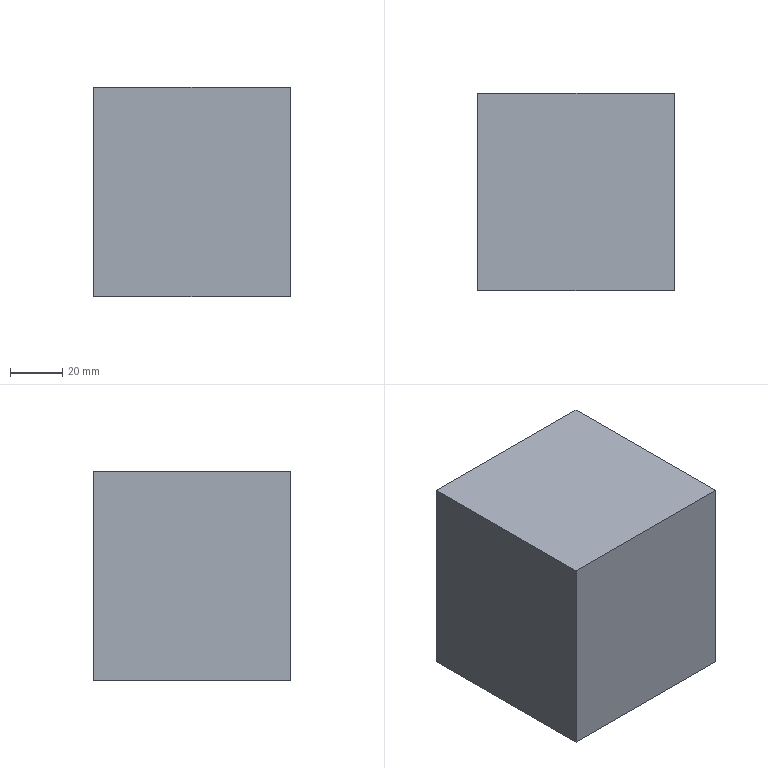Part | SolidWorks | features Extrusion 1, HoleWzd 1 | 1 solid | 30 faces | box 75 x 75 x 80 mm | volume 448174 mm3 | cylinder 12 | cone 12 | plane 6 | commonest cylinder face diameters 5 x12
STEP:
#1=CARTESIAN_POINT('',(34.,31.,15.));
#2=VERTEX_POINT('',#1);
#3=CARTESIAN_POINT('',(29.,31.,15.));
#4=VERTEX_POINT('',#3);
#5=CARTESIAN_POINT('',(31.5,31.,15.));
#6=DIRECTION('',(0.,0.,-1.));
#7=DIRECTION('',(-1.,0.,0.));
#8=AXIS2_PLACEMENT_3D('',#5,#6,#7);
#9=CIRCLE('',#8,2.5);
#10=EDGE_CURVE('',#2,#4,#9,.T.);
#11=ORIENTED_EDGE('',*,*,#10,.F.);
#12=CARTESIAN_POINT('',(34.,31.,0.));
#13=VERTEX_POINT('',#12);
#14=CARTESIAN_POINT('',(34.,31.,0.));
#15=DIRECTION('',(0.,0.,-1.));
#16=VECTOR('',#15,1000.);
#17=LINE('',#14,#16);
#18=EDGE_CURVE('',#2,#13,#17,.T.);
#19=ORIENTED_EDGE('',*,*,#18,.T.);
#20=CARTESIAN_POINT('',(29.,31.,0.));
#21=VERTEX_POINT('',#20);
#22=CARTESIAN_POINT('',(31.5,31.,0.));
#23=DIRECTION('',(0.,0.,-1.));
#24=DIRECTION('',(-1.,0.,0.));
#25=AXIS2_PLACEMENT_3D('',#22,#23,#24);
#26=CIRCLE('',#25,2.5);
#27=EDGE_CURVE('',#13,#21,#26,.T.);
#28=ORIENTED_EDGE('',*,*,#27,.T.);
#29=CARTESIAN_POINT('',(29.,31.,0.));
#30=DIRECTION('',(0.,0.,-1.));
#31=VECTOR('',#30,1000.);
#32=LINE('',#29,#31);
#33=EDGE_CURVE('',#4,#21,#32,.T.);
#34=ORIENTED_EDGE('',*,*,#33,.F.);
#35=EDGE_LOOP('',(#11,#19,#28,#34));
#36=FACE_OUTER_BOUND('',#35,.T.);
#37=CARTESIAN_POINT('',(31.5,31.,0.));
#38=DIRECTION('',(0.,0.,-1.));
#39=DIRECTION('',(-1.,0.,0.));
#40=AXIS2_PLACEMENT_3D('',#37,#38,#39);
#41=CYLINDRICAL_SURFACE('',#40,2.5);
#42=ADVANCED_FACE('',(#36),#41,.F.);
#43=CARTESIAN_POINT('',(31.5,31.,16.502));
#44=VERTEX_POINT('',#43);
#45=CARTESIAN_POINT('',(29.,31.,15.));
#46=DIRECTION('',(-0.8572,0.,-0.515));
#47=VECTOR('',#46,1000.);
#48=LINE('',#45,#47);
#49=EDGE_CURVE('',#44,#4,#48,.T.);
#50=ORIENTED_EDGE('',*,*,#49,.F.);
#51=CARTESIAN_POINT('',(34.,31.,15.));
#52=DIRECTION('',(0.8572,0.,-0.515));
#53=VECTOR('',#52,1000.);
#54=LINE('',#51,#53);
#55=EDGE_CURVE('',#44,#2,#54,.T.);
#56=ORIENTED_EDGE('',*,*,#55,.T.);
#57=ORIENTED_EDGE('',*,*,#10,.T.);
#58=EDGE_LOOP('',(#50,#56,#57));
#59=FACE_OUTER_BOUND('',#58,.T.);
#60=CARTESIAN_POINT('',(31.5,31.,15.));
#61=DIRECTION('',(0.,0.,-1.));
#62=DIRECTION('',(-1.,0.,0.));
#63=AXIS2_PLACEMENT_3D('',#60,#61,#62);
#64=CONICAL_SURFACE('',#63,2.5,1.03);
#65=ADVANCED_FACE('',(#59),#64,.F.);
#66=CARTESIAN_POINT('',(23.,31.,15.));
#67=VERTEX_POINT('',#66);
#68=CARTESIAN_POINT('',(18.,31.,15.));
#69=VERTEX_POINT('',#68);
#70=CARTESIAN_POINT('',(20.5,31.,15.));
#71=DIRECTION('',(0.,0.,-1.));
#72=DIRECTION('',(-1.,0.,0.));
#73=AXIS2_PLACEMENT_3D('',#70,#71,#72);
#74=CIRCLE('',#73,2.5);
#75=EDGE_CURVE('',#67,#69,#74,.T.);
#76=ORIENTED_EDGE('',*,*,#75,.F.);
#77=CARTESIAN_POINT('',(23.,31.,0.));
#78=VERTEX_POINT('',#77);
#79=CARTESIAN_POINT('',(23.,31.,0.));
#80=DIRECTION('',(0.,0.,-1.));
#81=VECTOR('',#80,1000.);
#82=LINE('',#79,#81);
#83=EDGE_CURVE('',#67,#78,#82,.T.);
#84=ORIENTED_EDGE('',*,*,#83,.T.);
#85=CARTESIAN_POINT('',(18.,31.,0.));
#86=VERTEX_POINT('',#85);
#87=CARTESIAN_POINT('',(20.5,31.,0.));
#88=DIRECTION('',(0.,0.,-1.));
#89=DIRECTION('',(-1.,0.,0.));
#90=AXIS2_PLACEMENT_3D('',#87,#88,#89);
#91=CIRCLE('',#90,2.5);
#92=EDGE_CURVE('',#78,#86,#91,.T.);
#93=ORIENTED_EDGE('',*,*,#92,.T.);
#94=CARTESIAN_POINT('',(18.,31.,0.));
#95=DIRECTION('',(0.,0.,-1.));
#96=VECTOR('',#95,1000.);
#97=LINE('',#94,#96);
#98=EDGE_CURVE('',#69,#86,#97,.T.);
#99=ORIENTED_EDGE('',*,*,#98,.F.);
#100=EDGE_LOOP('',(#76,#84,#93,#99));
#101=FACE_OUTER_BOUND('',#100,.T.);
#102=CARTESIAN_POINT('',(20.5,31.,0.));
#103=DIRECTION('',(0.,0.,-1.));
#104=DIRECTION('',(-1.,0.,0.));
#105=AXIS2_PLACEMENT_3D('',#102,#103,#104);
#106=CYLINDRICAL_SURFACE('',#105,2.5);
#107=ADVANCED_FACE('',(#101),#106,.F.);
#108=CARTESIAN_POINT('',(20.5,31.,16.502));
#109=VERTEX_POINT('',#108);
#110=CARTESIAN_POINT('',(18.,31.,15.));
#111=DIRECTION('',(-0.8572,0.,-0.515));
#112=VECTOR('',#111,1000.);
#113=LINE('',#110,#112);
#114=EDGE_CURVE('',#109,#69,#113,.T.);
#115=ORIENTED_EDGE('',*,*,#114,.F.);
#116=CARTESIAN_POINT('',(23.,31.,15.));
#117=DIRECTION('',(0.8572,0.,-0.515));
#118=VECTOR('',#117,1000.);
#119=LINE('',#116,#118);
#120=EDGE_CURVE('',#109,#67,#119,.T.);
#121=ORIENTED_EDGE('',*,*,#120,.T.);
#122=ORIENTED_EDGE('',*,*,#75,.T.);
#123=EDGE_LOOP('',(#115,#121,#122));
#124=FACE_OUTER_BOUND('',#123,.T.);
#125=CARTESIAN_POINT('',(20.5,31.,15.));
#126=DIRECTION('',(0.,0.,-1.));
#127=DIRECTION('',(-1.,0.,0.));
#128=AXIS2_PLACEMENT_3D('',#125,#126,#127);
#129=CONICAL_SURFACE('',#128,2.5,1.03);
#130=ADVANCED_FACE('',(#124),#129,.F.);
#131=CARTESIAN_POINT('',(-18.,31.,15.));
#132=VERTEX_POINT('',#131);
#133=CARTESIAN_POINT('',(-23.,31.,15.));
#134=VERTEX_POINT('',#133);
#135=CARTESIAN_POINT('',(-20.5,31.,15.));
#136=DIRECTION('',(0.,0.,-1.));
#137=DIRECTION('',(-1.,0.,0.));
#138=AXIS2_PLACEMENT_3D('',#135,#136,#137);
#139=CIRCLE('',#138,2.5);
#140=EDGE_CURVE('',#132,#134,#139,.T.);
#141=ORIENTED_EDGE('',*,*,#140,.F.);
#142=CARTESIAN_POINT('',(-18.,31.,0.));
#143=VERTEX_POINT('',#142);
#144=CARTESIAN_POINT('',(-18.,31.,0.));
#145=DIRECTION('',(0.,0.,-1.));
#146=VECTOR('',#145,1000.);
#147=LINE('',#144,#146);
#148=EDGE_CURVE('',#132,#143,#147,.T.);
#149=ORIENTED_EDGE('',*,*,#148,.T.);
#150=CARTESIAN_POINT('',(-23.,31.,0.));
#151=VERTEX_POINT('',#150);
#152=CARTESIAN_POINT('',(-20.5,31.,0.));
#153=DIRECTION('',(0.,0.,-1.));
#154=DIRECTION('',(-1.,0.,0.));
#155=AXIS2_PLACEMENT_3D('',#152,#153,#154);
#156=CIRCLE('',#155,2.5);
#157=EDGE_CURVE('',#143,#151,#156,.T.);
#158=ORIENTED_EDGE('',*,*,#157,.T.);
#159=CARTESIAN_POINT('',(-23.,31.,0.));
#160=DIRECTION('',(0.,0.,-1.));
#161=VECTOR('',#160,1000.);
#162=LINE('',#159,#161);
#163=EDGE_CURVE('',#134,#151,#162,.T.);
#164=ORIENTED_EDGE('',*,*,#163,.F.);
#165=EDGE_LOOP('',(#141,#149,#158,#164));
#166=FACE_OUTER_BOUND('',#165,.T.);
#167=CARTESIAN_POINT('',(-20.5,31.,0.));
#168=DIRECTION('',(0.,0.,-1.));
#169=DIRECTION('',(-1.,0.,0.));
#170=AXIS2_PLACEMENT_3D('',#167,#168,#169);
#171=CYLINDRICAL_SURFACE('',#170,2.5);
#172=ADVANCED_FACE('',(#166),#171,.F.);
#173=CARTESIAN_POINT('',(-20.5,31.,16.502));
#174=VERTEX_POINT('',#173);
#175=CARTESIAN_POINT('',(-23.,31.,15.));
#176=DIRECTION('',(-0.8572,0.,-0.515));
#177=VECTOR('',#176,1000.);
#178=LINE('',#175,#177);
#179=EDGE_CURVE('',#174,#134,#178,.T.);
#180=ORIENTED_EDGE('',*,*,#179,.F.);
#181=CARTESIAN_POINT('',(-18.,31.,15.));
#182=DIRECTION('',(0.8572,0.,-0.515));
#183=VECTOR('',#182,1000.);
#184=LINE('',#181,#183);
#185=EDGE_CURVE('',#174,#132,#184,.T.);
#186=ORIENTED_EDGE('',*,*,#185,.T.);
#187=ORIENTED_EDGE('',*,*,#140,.T.);
#188=EDGE_LOOP('',(#180,#186,#187));
#189=FACE_OUTER_BOUND('',#188,.T.);
#190=CARTESIAN_POINT('',(-20.5,31.,15.));
#191=DIRECTION('',(0.,0.,-1.));
#192=DIRECTION('',(-1.,0.,0.));
#193=AXIS2_PLACEMENT_3D('',#190,#191,#192);
#194=CONICAL_SURFACE('',#193,2.5,1.03);
#195=ADVANCED_FACE('',(#189),#194,.F.);
#196=CARTESIAN_POINT('',(-18.,-31.,15.));
#197=VERTEX_POINT('',#196);
#198=CARTESIAN_POINT('',(-23.,-31.,15.));
#199=VERTEX_POINT('',#198);
#200=CARTESIAN_POINT('',(-20.5,-31.,15.));
#201=DIRECTION('',(0.,0.,-1.));
#202=DIRECTION('',(-1.,0.,0.));
#203=AXIS2_PLACEMENT_3D('',#200,#201,#202);
#204=CIRCLE('',#203,2.5);
#205=EDGE_CURVE('',#197,#199,#204,.T.);
#206=ORIENTED_EDGE('',*,*,#205,.F.);
#207=CARTESIAN_POINT('',(-18.,-31.,0.));
#208=VERTEX_POINT('',#207);
#209=CARTESIAN_POINT('',(-18.,-31.,0.));
#210=DIRECTION('',(0.,0.,-1.));
#211=VECTOR('',#210,1000.);
#212=LINE('',#209,#211);
#213=EDGE_CURVE('',#197,#208,#212,.T.);
#214=ORIENTED_EDGE('',*,*,#213,.T.);
#215=CARTESIAN_POINT('',(-23.,-31.,0.));
#216=VERTEX_POINT('',#215);
#217=CARTESIAN_POINT('',(-20.5,-31.,0.));
#218=DIRECTION('',(0.,0.,-1.));
#219=DIRECTION('',(-1.,0.,0.));
#220=AXIS2_PLACEMENT_3D('',#217,#218,#219);
#221=CIRCLE('',#220,2.5);
#222=EDGE_CURVE('',#208,#216,#221,.T.);
#223=ORIENTED_EDGE('',*,*,#222,.T.);
#224=CARTESIAN_POINT('',(-23.,-31.,0.));
#225=DIRECTION('',(0.,0.,-1.));
#226=VECTOR('',#225,1000.);
#227=LINE('',#224,#226);
#228=EDGE_CURVE('',#199,#216,#227,.T.);
#229=ORIENTED_EDGE('',*,*,#228,.F.);
#230=EDGE_LOOP('',(#206,#214,#223,#229));
#231=FACE_OUTER_BOUND('',#230,.T.);
#232=CARTESIAN_POINT('',(-20.5,-31.,0.));
#233=DIRECTION('',(0.,0.,-1.));
#234=DIRECTION('',(-1.,0.,0.));
#235=AXIS2_PLACEMENT_3D('',#232,#233,#234);
#236=CYLINDRICAL_SURFACE('',#235,2.5);
#237=ADVANCED_FACE('',(#231),#236,.F.);
#238=CARTESIAN_POINT('',(-20.5,-31.,16.502));
#239=VERTEX_POINT('',#238);
#240=CARTESIAN_POINT('',(-23.,-31.,15.));
#241=DIRECTION('',(-0.8572,0.,-0.515));
#242=VECTOR('',#241,1000.);
#243=LINE('',#240,#242);
#244=EDGE_CURVE('',#239,#199,#243,.T.);
#245=ORIENTED_EDGE('',*,*,#244,.F.);
#246=CARTESIAN_POINT('',(-18.,-31.,15.));
#247=DIRECTION('',(0.8572,0.,-0.515));
#248=VECTOR('',#247,1000.);
#249=LINE('',#246,#248);
#250=EDGE_CURVE('',#239,#197,#249,.T.);
#251=ORIENTED_EDGE('',*,*,#250,.T.);
#252=ORIENTED_EDGE('',*,*,#205,.T.);
#253=EDGE_LOOP('',(#245,#251,#252));
#254=FACE_OUTER_BOUND('',#253,.T.);
#255=CARTESIAN_POINT('',(-20.5,-31.,15.));
#256=DIRECTION('',(0.,0.,-1.));
#257=DIRECTION('',(-1.,0.,0.));
#258=AXIS2_PLACEMENT_3D('',#255,#256,#257);
#259=CONICAL_SURFACE('',#258,2.5,1.03);
#260=ADVANCED_FACE('',(#254),#259,.F.);
#261=CARTESIAN_POINT('',(23.,-31.,15.));
#262=VERTEX_POINT('',#261);
#263=CARTESIAN_POINT('',(18.,-31.,15.));
#264=VERTEX_POINT('',#263);
#265=CARTESIAN_POINT('',(20.5,-31.,15.));
#266=DIRECTION('',(0.,0.,-1.));
#267=DIRECTION('',(-1.,0.,0.));
#268=AXIS2_PLACEMENT_3D('',#265,#266,#267);
#269=CIRCLE('',#268,2.5);
#270=EDGE_CURVE('',#262,#264,#269,.T.);
#271=ORIENTED_EDGE('',*,*,#270,.F.);
#272=CARTESIAN_POINT('',(23.,-31.,0.));
#273=VERTEX_POINT('',#272);
#274=CARTESIAN_POINT('',(23.,-31.,0.));
#275=DIRECTION('',(0.,0.,-1.));
#276=VECTOR('',#275,1000.);
#277=LINE('',#274,#276);
#278=EDGE_CURVE('',#262,#273,#277,.T.);
#279=ORIENTED_EDGE('',*,*,#278,.T.);
#280=CARTESIAN_POINT('',(18.,-31.,0.));
#281=VERTEX_POINT('',#280);
#282=CARTESIAN_POINT('',(20.5,-31.,0.));
#283=DIRECTION('',(0.,0.,-1.));
#284=DIRECTION('',(-1.,0.,0.));
#285=AXIS2_PLACEMENT_3D('',#282,#283,#284);
#286=CIRCLE('',#285,2.5);
#287=EDGE_CURVE('',#273,#281,#286,.T.);
#288=ORIENTED_EDGE('',*,*,#287,.T.);
#289=CARTESIAN_POINT('',(18.,-31.,0.));
#290=DIRECTION('',(0.,0.,-1.));
#291=VECTOR('',#290,1000.);
#292=LINE('',#289,#291);
#293=EDGE_CURVE('',#264,#281,#292,.T.);
#294=ORIENTED_EDGE('',*,*,#293,.F.);
#295=EDGE_LOOP('',(#271,#279,#288,#294));
#296=FACE_OUTER_BOUND('',#295,.T.);
#297=CARTESIAN_POINT('',(20.5,-31.,0.));
#298=DIRECTION('',(0.,0.,-1.));
#299=DIRECTION('',(-1.,0.,0.));
#300=AXIS2_PLACEMENT_3D('',#297,#298,#299);
#301=CYLINDRICAL_SURFACE('',#300,2.5);
#302=ADVANCED_FACE('',(#296),#301,.F.);
#303=CARTESIAN_POINT('',(20.5,-31.,16.502));
#304=VERTEX_POINT('',#303);
#305=CARTESIAN_POINT('',(18.,-31.,15.));
#306=DIRECTION('',(-0.8572,0.,-0.515));
#307=VECTOR('',#306,1000.);
#308=LINE('',#305,#307);
#309=EDGE_CURVE('',#304,#264,#308,.T.);
#310=ORIENTED_EDGE('',*,*,#309,.F.);
#311=CARTESIAN_POINT('',(23.,-31.,15.));
#312=DIRECTION('',(0.8572,0.,-0.515));
#313=VECTOR('',#312,1000.);
#314=LINE('',#311,#313);
#315=EDGE_CURVE('',#304,#262,#314,.T.);
#316=ORIENTED_EDGE('',*,*,#315,.T.);
#317=ORIENTED_EDGE('',*,*,#270,.T.);
#318=EDGE_LOOP('',(#310,#316,#317));
#319=FACE_OUTER_BOUND('',#318,.T.);
#320=CARTESIAN_POINT('',(20.5,-31.,15.));
#321=DIRECTION('',(0.,0.,-1.));
#322=DIRECTION('',(-1.,0.,0.));
#323=AXIS2_PLACEMENT_3D('',#320,#321,#322);
#324=CONICAL_SURFACE('',#323,2.5,1.03);
#325=ADVANCED_FACE('',(#319),#324,.F.);
#326=CARTESIAN_POINT('',(34.,-31.,15.));
#327=VERTEX_POINT('',#326);
#328=CARTESIAN_POINT('',(29.,-31.,15.));
#329=VERTEX_POINT('',#328);
#330=CARTESIAN_POINT('',(31.5,-31.,15.));
#331=DIRECTION('',(0.,0.,-1.));
#332=DIRECTION('',(-1.,0.,0.));
#333=AXIS2_PLACEMENT_3D('',#330,#331,#332);
#334=CIRCLE('',#333,2.5);
#335=EDGE_CURVE('',#327,#329,#334,.T.);
#336=ORIENTED_EDGE('',*,*,#335,.F.);
#337=CARTESIAN_POINT('',(34.,-31.,0.));
#338=VERTEX_POINT('',#337);
#339=CARTESIAN_POINT('',(34.,-31.,0.));
#340=DIRECTION('',(0.,0.,-1.));
#341=VECTOR('',#340,1000.);
#342=LINE('',#339,#341);
#343=EDGE_CURVE('',#327,#338,#342,.T.);
#344=ORIENTED_EDGE('',*,*,#343,.T.);
#345=CARTESIAN_POINT('',(29.,-31.,0.));
#346=VERTEX_POINT('',#345);
#347=CARTESIAN_POINT('',(31.5,-31.,0.));
#348=DIRECTION('',(0.,0.,-1.));
#349=DIRECTION('',(-1.,0.,0.));
#350=AXIS2_PLACEMENT_3D('',#347,#348,#349);
#351=CIRCLE('',#350,2.5);
#352=EDGE_CURVE('',#338,#346,#351,.T.);
#353=ORIENTED_EDGE('',*,*,#352,.T.);
#354=CARTESIAN_POINT('',(29.,-31.,0.));
#355=DIRECTION('',(0.,0.,-1.));
#356=VECTOR('',#355,1000.);
#357=LINE('',#354,#356);
#358=EDGE_CURVE('',#329,#346,#357,.T.);
#359=ORIENTED_EDGE('',*,*,#358,.F.);
#360=EDGE_LOOP('',(#336,#344,#353,#359));
#361=FACE_OUTER_BOUND('',#360,.T.);
#362=CARTESIAN_POINT('',(31.5,-31.,0.));
#363=DIRECTION('',(0.,0.,-1.));
#364=DIRECTION('',(-1.,0.,0.));
#365=AXIS2_PLACEMENT_3D('',#362,#363,#364);
#366=CYLINDRICAL_SURFACE('',#365,2.5);
#367=ADVANCED_FACE('',(#361),#366,.F.);
#368=CARTESIAN_POINT('',(31.5,-31.,16.502));
#369=VERTEX_POINT('',#368);
#370=CARTESIAN_POINT('',(29.,-31.,15.));
#371=DIRECTION('',(-0.8572,0.,-0.515));
#372=VECTOR('',#371,1000.);
#373=LINE('',#370,#372);
#374=EDGE_CURVE('',#369,#329,#373,.T.);
#375=ORIENTED_EDGE('',*,*,#374,.F.);
#376=CARTESIAN_POINT('',(34.,-31.,15.));
#377=DIRECTION('',(0.8572,0.,-0.515));
#378=VECTOR('',#377,1000.);
#379=LINE('',#376,#378);
#380=EDGE_CURVE('',#369,#327,#379,.T.);
#381=ORIENTED_EDGE('',*,*,#380,.T.);
#382=ORIENTED_EDGE('',*,*,#335,.T.);
#383=EDGE_LOOP('',(#375,#381,#382));
#384=FACE_OUTER_BOUND('',#383,.T.);
#385=CARTESIAN_POINT('',(31.5,-31.,15.));
#386=DIRECTION('',(0.,0.,-1.));
#387=DIRECTION('',(-1.,0.,0.));
#388=AXIS2_PLACEMENT_3D('',#385,#386,#387);
#389=CONICAL_SURFACE('',#388,2.5,1.03);
#390=ADVANCED_FACE('',(#384),#389,.F.);
#391=CARTESIAN_POINT('',(37.5,-37.5,0.));
#392=VERTEX_POINT('',#391);
#393=CARTESIAN_POINT('',(37.5,37.5,0.));
#394=VERTEX_POINT('',#393);
#395=CARTESIAN_POINT('',(37.5,37.5,0.));
#396=DIRECTION('',(0.,1.,0.));
#397=VECTOR('',#396,1000.);
#398=LINE('',#395,#397);
#399=EDGE_CURVE('',#392,#394,#398,.T.);
#400=ORIENTED_EDGE('',*,*,#399,.T.);
#401=CARTESIAN_POINT('',(37.5,37.5,80.));
#402=VERTEX_POINT('',#401);
#403=CARTESIAN_POINT('',(37.5,37.5,80.));
#404=DIRECTION('',(0.,0.,-1.));
#405=VECTOR('',#404,1000.);
#406=LINE('',#403,#405);
#407=EDGE_CURVE('',#402,#394,#406,.T.);
#408=ORIENTED_EDGE('',*,*,#407,.F.);
#409=CARTESIAN_POINT('',(37.5,-37.5,80.));
#410=VERTEX_POINT('',#409);
#411=CARTESIAN_POINT('',(37.5,37.5,80.));
#412=DIRECTION('',(0.,1.,0.));
#413=VECTOR('',#412,1000.);
#414=LINE('',#411,#413);
#415=EDGE_CURVE('',#410,#402,#414,.T.);
#416=ORIENTED_EDGE('',*,*,#415,.F.);
#417=CARTESIAN_POINT('',(37.5,-37.5,80.));
#418=DIRECTION('',(0.,0.,-1.));
#419=VECTOR('',#418,1000.);
#420=LINE('',#417,#419);
#421=EDGE_CURVE('',#410,#392,#420,.T.);
#422=ORIENTED_EDGE('',*,*,#421,.T.);
#423=EDGE_LOOP('',(#400,#408,#416,#422));
#424=FACE_OUTER_BOUND('',#423,.T.);
#425=CARTESIAN_POINT('',(37.5,37.5,80.));
#426=DIRECTION('',(-1.,0.,0.));
#427=DIRECTION('',(0.,-1.,0.));
#428=AXIS2_PLACEMENT_3D('',#425,#426,#427);
#429=PLANE('',#428);
#430=ADVANCED_FACE('',(#424),#429,.F.);
#431=CARTESIAN_POINT('',(-37.5,37.5,0.));
#432=VERTEX_POINT('',#431);
#433=CARTESIAN_POINT('',(-37.5,37.5,0.));
#434=DIRECTION('',(-1.,0.,0.));
#435=VECTOR('',#434,1000.);
#436=LINE('',#433,#435);
#437=EDGE_CURVE('',#394,#432,#436,.T.);
#438=ORIENTED_EDGE('',*,*,#437,.T.);
#439=CARTESIAN_POINT('',(-37.5,37.5,80.));
#440=VERTEX_POINT('',#439);
#441=CARTESIAN_POINT('',(-37.5,37.5,80.));
#442=DIRECTION('',(0.,0.,-1.));
#443=VECTOR('',#442,1000.);
#444=LINE('',#441,#443);
#445=EDGE_CURVE('',#440,#432,#444,.T.);
#446=ORIENTED_EDGE('',*,*,#445,.F.);
#447=CARTESIAN_POINT('',(-37.5,37.5,80.));
#448=DIRECTION('',(-1.,0.,0.));
#449=VECTOR('',#448,1000.);
#450=LINE('',#447,#449);
#451=EDGE_CURVE('',#402,#440,#450,.T.);
#452=ORIENTED_EDGE('',*,*,#451,.F.);
#453=ORIENTED_EDGE('',*,*,#407,.T.);
#454=EDGE_LOOP('',(#438,#446,#452,#453));
#455=FACE_OUTER_BOUND('',#454,.T.);
#456=CARTESIAN_POINT('',(-37.5,37.5,80.));
#457=DIRECTION('',(0.,-1.,0.));
#458=DIRECTION('',(0.,0.,-1.));
#459=AXIS2_PLACEMENT_3D('',#456,#457,#458);
#460=PLANE('',#459);
#461=ADVANCED_FACE('',(#455),#460,.F.);
#462=CARTESIAN_POINT('',(-37.5,-37.5,0.));
#463=VERTEX_POINT('',#462);
#464=CARTESIAN_POINT('',(-37.5,37.5,0.));
#465=DIRECTION('',(0.,-1.,0.));
#466=VECTOR('',#465,1000.);
#467=LINE('',#464,#466);
#468=EDGE_CURVE('',#432,#463,#467,.T.);
#469=ORIENTED_EDGE('',*,*,#468,.T.);
#470=CARTESIAN_POINT('',(-37.5,-37.5,80.));
#471=VERTEX_POINT('',#470);
#472=CARTESIAN_POINT('',(-37.5,-37.5,80.));
#473=DIRECTION('',(0.,0.,-1.));
#474=VECTOR('',#473,1000.);
#475=LINE('',#472,#474);
#476=EDGE_CURVE('',#471,#463,#475,.T.);
#477=ORIENTED_EDGE('',*,*,#476,.F.);
#478=CARTESIAN_POINT('',(-37.5,37.5,80.));
#479=DIRECTION('',(0.,-1.,0.));
#480=VECTOR('',#479,1000.);
#481=LINE('',#478,#480);
#482=EDGE_CURVE('',#440,#471,#481,.T.);
#483=ORIENTED_EDGE('',*,*,#482,.F.);
#484=ORIENTED_EDGE('',*,*,#445,.T.);
#485=EDGE_LOOP('',(#469,#477,#483,#484));
#486=FACE_OUTER_BOUND('',#485,.T.);
#487=CARTESIAN_POINT('',(-37.5,37.5,80.));
#488=DIRECTION('',(1.,0.,0.));
#489=DIRECTION('',(0.,1.,0.));
#490=AXIS2_PLACEMENT_3D('',#487,#488,#489);
#491=PLANE('',#490);
#492=ADVANCED_FACE('',(#486),#491,.F.);
#493=CARTESIAN_POINT('',(-37.5,-37.5,0.));
#494=DIRECTION('',(1.,0.,0.));
#495=VECTOR('',#494,1000.);
#496=LINE('',#493,#495);
#497=EDGE_CURVE('',#463,#392,#496,.T.);
#498=ORIENTED_EDGE('',*,*,#497,.T.);
#499=ORIENTED_EDGE('',*,*,#421,.F.);
#500=CARTESIAN_POINT('',(-37.5,-37.5,80.));
#501=DIRECTION('',(1.,0.,0.));
#502=VECTOR('',#501,1000.);
#503=LINE('',#500,#502);
#504=EDGE_CURVE('',#471,#410,#503,.T.);
#505=ORIENTED_EDGE('',*,*,#504,.F.);
#506=ORIENTED_EDGE('',*,*,#476,.T.);
#507=EDGE_LOOP('',(#498,#499,#505,#506));
#508=FACE_OUTER_BOUND('',#507,.T.);
#509=CARTESIAN_POINT('',(-37.5,-37.5,80.));
#510=DIRECTION('',(0.,1.,0.));
#511=DIRECTION('',(0.,0.,1.));
#512=AXIS2_PLACEMENT_3D('',#509,#510,#511);
#513=PLANE('',#512);
#514=ADVANCED_FACE('',(#508),#513,.F.);
#515=ORIENTED_EDGE('',*,*,#415,.T.);
#516=ORIENTED_EDGE('',*,*,#451,.T.);
#517=ORIENTED_EDGE('',*,*,#482,.T.);
#518=ORIENTED_EDGE('',*,*,#504,.T.);
#519=EDGE_LOOP('',(#515,#516,#517,#518));
#520=FACE_OUTER_BOUND('',#519,.T.);
#521=CARTESIAN_POINT('',(0.,0.,80.));
#522=DIRECTION('',(0.,0.,1.));
#523=DIRECTION('',(1.,0.,0.));
#524=AXIS2_PLACEMENT_3D('',#521,#522,#523);
#525=PLANE('',#524);
#526=ADVANCED_FACE('',(#520),#525,.T.);
#527=CARTESIAN_POINT('',(31.5,31.,0.));
#528=DIRECTION('',(0.,0.,-1.));
#529=DIRECTION('',(-1.,0.,0.));
#530=AXIS2_PLACEMENT_3D('',#527,#528,#529);
#531=CIRCLE('',#530,2.5);
#532=EDGE_CURVE('',#21,#13,#531,.T.);
#533=ORIENTED_EDGE('',*,*,#532,.F.);
#534=ORIENTED_EDGE('',*,*,#27,.F.);
#535=EDGE_LOOP('',(#533,#534));
#536=FACE_BOUND('',#535,.T.);
#537=CARTESIAN_POINT('',(20.5,31.,0.));
#538=DIRECTION('',(0.,0.,-1.));
#539=DIRECTION('',(-1.,0.,0.));
#540=AXIS2_PLACEMENT_3D('',#537,#538,#539);
#541=CIRCLE('',#540,2.5);
#542=EDGE_CURVE('',#86,#78,#541,.T.);
#543=ORIENTED_EDGE('',*,*,#542,.F.);
#544=ORIENTED_EDGE('',*,*,#92,.F.);
#545=EDGE_LOOP('',(#543,#544));
#546=FACE_BOUND('',#545,.T.);
#547=CARTESIAN_POINT('',(-20.5,31.,0.));
#548=DIRECTION('',(0.,0.,-1.));
#549=DIRECTION('',(-1.,0.,0.));
#550=AXIS2_PLACEMENT_3D('',#547,#548,#549);
#551=CIRCLE('',#550,2.5);
#552=EDGE_CURVE('',#151,#143,#551,.T.);
#553=ORIENTED_EDGE('',*,*,#552,.F.);
#554=ORIENTED_EDGE('',*,*,#157,.F.);
#555=EDGE_LOOP('',(#553,#554));
#556=FACE_BOUND('',#555,.T.);
#557=CARTESIAN_POINT('',(-20.5,-31.,0.));
#558=DIRECTION('',(0.,0.,-1.));
#559=DIRECTION('',(-1.,0.,0.));
#560=AXIS2_PLACEMENT_3D('',#557,#558,#559);
#561=CIRCLE('',#560,2.5);
#562=EDGE_CURVE('',#216,#208,#561,.T.);
#563=ORIENTED_EDGE('',*,*,#562,.F.);
#564=ORIENTED_EDGE('',*,*,#222,.F.);
#565=EDGE_LOOP('',(#563,#564));
#566=FACE_BOUND('',#565,.T.);
#567=CARTESIAN_POINT('',(20.5,-31.,0.));
#568=DIRECTION('',(0.,0.,-1.));
#569=DIRECTION('',(-1.,0.,0.));
#570=AXIS2_PLACEMENT_3D('',#567,#568,#569);
#571=CIRCLE('',#570,2.5);
#572=EDGE_CURVE('',#281,#273,#571,.T.);
#573=ORIENTED_EDGE('',*,*,#572,.F.);
#574=ORIENTED_EDGE('',*,*,#287,.F.);
#575=EDGE_LOOP('',(#573,#574));
#576=FACE_BOUND('',#575,.T.);
#577=CARTESIAN_POINT('',(31.5,-31.,0.));
#578=DIRECTION('',(0.,0.,-1.));
#579=DIRECTION('',(-1.,0.,0.));
#580=AXIS2_PLACEMENT_3D('',#577,#578,#579);
#581=CIRCLE('',#580,2.5);
#582=EDGE_CURVE('',#346,#338,#581,.T.);
#583=ORIENTED_EDGE('',*,*,#582,.F.);
#584=ORIENTED_EDGE('',*,*,#352,.F.);
#585=EDGE_LOOP('',(#583,#584));
#586=FACE_BOUND('',#585,.T.);
#587=ORIENTED_EDGE('',*,*,#399,.F.);
#588=ORIENTED_EDGE('',*,*,#497,.F.);
#589=ORIENTED_EDGE('',*,*,#468,.F.);
#590=ORIENTED_EDGE('',*,*,#437,.F.);
#591=EDGE_LOOP('',(#587,#588,#589,#590));
#592=FACE_OUTER_BOUND('',#591,.T.);
#593=CARTESIAN_POINT('',(0.,0.,0.));
#594=DIRECTION('',(0.,0.,1.));
#595=DIRECTION('',(1.,0.,0.));
#596=AXIS2_PLACEMENT_3D('',#593,#594,#595);
#597=PLANE('',#596);
#598=ADVANCED_FACE('',(#536,#546,#556,#566,#576,#586,#592),#597,.F.);
#599=ORIENTED_EDGE('',*,*,#380,.F.);
#600=ORIENTED_EDGE('',*,*,#374,.T.);
#601=CARTESIAN_POINT('',(31.5,-31.,15.));
#602=DIRECTION('',(0.,0.,-1.));
#603=DIRECTION('',(-1.,0.,0.));
#604=AXIS2_PLACEMENT_3D('',#601,#602,#603);
#605=CIRCLE('',#604,2.5);
#606=EDGE_CURVE('',#329,#327,#605,.T.);
#607=ORIENTED_EDGE('',*,*,#606,.T.);
#608=EDGE_LOOP('',(#599,#600,#607));
#609=FACE_OUTER_BOUND('',#608,.T.);
#610=CARTESIAN_POINT('',(31.5,-31.,15.));
#611=DIRECTION('',(0.,0.,-1.));
#612=DIRECTION('',(-1.,0.,0.));
#613=AXIS2_PLACEMENT_3D('',#610,#611,#612);
#614=CONICAL_SURFACE('',#613,2.5,1.03);
#615=ADVANCED_FACE('',(#609),#614,.F.);
#616=ORIENTED_EDGE('',*,*,#343,.F.);
#617=ORIENTED_EDGE('',*,*,#606,.F.);
#618=ORIENTED_EDGE('',*,*,#358,.T.);
#619=ORIENTED_EDGE('',*,*,#582,.T.);
#620=EDGE_LOOP('',(#616,#617,#618,#619));
#621=FACE_OUTER_BOUND('',#620,.T.);
#622=CARTESIAN_POINT('',(31.5,-31.,0.));
#623=DIRECTION('',(0.,0.,-1.));
#624=DIRECTION('',(-1.,0.,0.));
#625=AXIS2_PLACEMENT_3D('',#622,#623,#624);
#626=CYLINDRICAL_SURFACE('',#625,2.5);
#627=ADVANCED_FACE('',(#621),#626,.F.);
#628=ORIENTED_EDGE('',*,*,#315,.F.);
#629=ORIENTED_EDGE('',*,*,#309,.T.);
#630=CARTESIAN_POINT('',(20.5,-31.,15.));
#631=DIRECTION('',(0.,0.,-1.));
#632=DIRECTION('',(-1.,0.,0.));
#633=AXIS2_PLACEMENT_3D('',#630,#631,#632);
#634=CIRCLE('',#633,2.5);
#635=EDGE_CURVE('',#264,#262,#634,.T.);
#636=ORIENTED_EDGE('',*,*,#635,.T.);
#637=EDGE_LOOP('',(#628,#629,#636));
#638=FACE_OUTER_BOUND('',#637,.T.);
#639=CARTESIAN_POINT('',(20.5,-31.,15.));
#640=DIRECTION('',(0.,0.,-1.));
#641=DIRECTION('',(-1.,0.,0.));
#642=AXIS2_PLACEMENT_3D('',#639,#640,#641);
#643=CONICAL_SURFACE('',#642,2.5,1.03);
#644=ADVANCED_FACE('',(#638),#643,.F.);
#645=ORIENTED_EDGE('',*,*,#278,.F.);
#646=ORIENTED_EDGE('',*,*,#635,.F.);
#647=ORIENTED_EDGE('',*,*,#293,.T.);
#648=ORIENTED_EDGE('',*,*,#572,.T.);
#649=EDGE_LOOP('',(#645,#646,#647,#648));
#650=FACE_OUTER_BOUND('',#649,.T.);
#651=CARTESIAN_POINT('',(20.5,-31.,0.));
#652=DIRECTION('',(0.,0.,-1.));
#653=DIRECTION('',(-1.,0.,0.));
#654=AXIS2_PLACEMENT_3D('',#651,#652,#653);
#655=CYLINDRICAL_SURFACE('',#654,2.5);
#656=ADVANCED_FACE('',(#650),#655,.F.);
#657=ORIENTED_EDGE('',*,*,#250,.F.);
#658=ORIENTED_EDGE('',*,*,#244,.T.);
#659=CARTESIAN_POINT('',(-20.5,-31.,15.));
#660=DIRECTION('',(0.,0.,-1.));
#661=DIRECTION('',(-1.,0.,0.));
#662=AXIS2_PLACEMENT_3D('',#659,#660,#661);
#663=CIRCLE('',#662,2.5);
#664=EDGE_CURVE('',#199,#197,#663,.T.);
#665=ORIENTED_EDGE('',*,*,#664,.T.);
#666=EDGE_LOOP('',(#657,#658,#665));
#667=FACE_OUTER_BOUND('',#666,.T.);
#668=CARTESIAN_POINT('',(-20.5,-31.,15.));
#669=DIRECTION('',(0.,0.,-1.));
#670=DIRECTION('',(-1.,0.,0.));
#671=AXIS2_PLACEMENT_3D('',#668,#669,#670);
#672=CONICAL_SURFACE('',#671,2.5,1.03);
#673=ADVANCED_FACE('',(#667),#672,.F.);
#674=ORIENTED_EDGE('',*,*,#213,.F.);
#675=ORIENTED_EDGE('',*,*,#664,.F.);
#676=ORIENTED_EDGE('',*,*,#228,.T.);
#677=ORIENTED_EDGE('',*,*,#562,.T.);
#678=EDGE_LOOP('',(#674,#675,#676,#677));
#679=FACE_OUTER_BOUND('',#678,.T.);
#680=CARTESIAN_POINT('',(-20.5,-31.,0.));
#681=DIRECTION('',(0.,0.,-1.));
#682=DIRECTION('',(-1.,0.,0.));
#683=AXIS2_PLACEMENT_3D('',#680,#681,#682);
#684=CYLINDRICAL_SURFACE('',#683,2.5);
#685=ADVANCED_FACE('',(#679),#684,.F.);
#686=ORIENTED_EDGE('',*,*,#185,.F.);
#687=ORIENTED_EDGE('',*,*,#179,.T.);
#688=CARTESIAN_POINT('',(-20.5,31.,15.));
#689=DIRECTION('',(0.,0.,-1.));
#690=DIRECTION('',(-1.,0.,0.));
#691=AXIS2_PLACEMENT_3D('',#688,#689,#690);
#692=CIRCLE('',#691,2.5);
#693=EDGE_CURVE('',#134,#132,#692,.T.);
#694=ORIENTED_EDGE('',*,*,#693,.T.);
#695=EDGE_LOOP('',(#686,#687,#694));
#696=FACE_OUTER_BOUND('',#695,.T.);
#697=CARTESIAN_POINT('',(-20.5,31.,15.));
#698=DIRECTION('',(0.,0.,-1.));
#699=DIRECTION('',(-1.,0.,0.));
#700=AXIS2_PLACEMENT_3D('',#697,#698,#699);
#701=CONICAL_SURFACE('',#700,2.5,1.03);
#702=ADVANCED_FACE('',(#696),#701,.F.);
#703=ORIENTED_EDGE('',*,*,#148,.F.);
#704=ORIENTED_EDGE('',*,*,#693,.F.);
#705=ORIENTED_EDGE('',*,*,#163,.T.);
#706=ORIENTED_EDGE('',*,*,#552,.T.);
#707=EDGE_LOOP('',(#703,#704,#705,#706));
#708=FACE_OUTER_BOUND('',#707,.T.);
#709=CARTESIAN_POINT('',(-20.5,31.,0.));
#710=DIRECTION('',(0.,0.,-1.));
#711=DIRECTION('',(-1.,0.,0.));
#712=AXIS2_PLACEMENT_3D('',#709,#710,#711);
#713=CYLINDRICAL_SURFACE('',#712,2.5);
#714=ADVANCED_FACE('',(#708),#713,.F.);
#715=ORIENTED_EDGE('',*,*,#120,.F.);
#716=ORIENTED_EDGE('',*,*,#114,.T.);
#717=CARTESIAN_POINT('',(20.5,31.,15.));
#718=DIRECTION('',(0.,0.,-1.));
#719=DIRECTION('',(-1.,0.,0.));
#720=AXIS2_PLACEMENT_3D('',#717,#718,#719);
#721=CIRCLE('',#720,2.5);
#722=EDGE_CURVE('',#69,#67,#721,.T.);
#723=ORIENTED_EDGE('',*,*,#722,.T.);
#724=EDGE_LOOP('',(#715,#716,#723));
#725=FACE_OUTER_BOUND('',#724,.T.);
#726=CARTESIAN_POINT('',(20.5,31.,15.));
#727=DIRECTION('',(0.,0.,-1.));
#728=DIRECTION('',(-1.,0.,0.));
#729=AXIS2_PLACEMENT_3D('',#726,#727,#728);
#730=CONICAL_SURFACE('',#729,2.5,1.03);
#731=ADVANCED_FACE('',(#725),#730,.F.);
#732=ORIENTED_EDGE('',*,*,#83,.F.);
#733=ORIENTED_EDGE('',*,*,#722,.F.);
#734=ORIENTED_EDGE('',*,*,#98,.T.);
#735=ORIENTED_EDGE('',*,*,#542,.T.);
#736=EDGE_LOOP('',(#732,#733,#734,#735));
#737=FACE_OUTER_BOUND('',#736,.T.);
#738=CARTESIAN_POINT('',(20.5,31.,0.));
#739=DIRECTION('',(0.,0.,-1.));
#740=DIRECTION('',(-1.,0.,0.));
#741=AXIS2_PLACEMENT_3D('',#738,#739,#740);
#742=CYLINDRICAL_SURFACE('',#741,2.5);
#743=ADVANCED_FACE('',(#737),#742,.F.);
#744=ORIENTED_EDGE('',*,*,#55,.F.);
#745=ORIENTED_EDGE('',*,*,#49,.T.);
#746=CARTESIAN_POINT('',(31.5,31.,15.));
#747=DIRECTION('',(0.,0.,-1.));
#748=DIRECTION('',(-1.,0.,0.));
#749=AXIS2_PLACEMENT_3D('',#746,#747,#748);
#750=CIRCLE('',#749,2.5);
#751=EDGE_CURVE('',#4,#2,#750,.T.);
#752=ORIENTED_EDGE('',*,*,#751,.T.);
#753=EDGE_LOOP('',(#744,#745,#752));
#754=FACE_OUTER_BOUND('',#753,.T.);
#755=CARTESIAN_POINT('',(31.5,31.,15.));
#756=DIRECTION('',(0.,0.,-1.));
#757=DIRECTION('',(-1.,0.,0.));
#758=AXIS2_PLACEMENT_3D('',#755,#756,#757);
#759=CONICAL_SURFACE('',#758,2.5,1.03);
#760=ADVANCED_FACE('',(#754),#759,.F.);
#761=ORIENTED_EDGE('',*,*,#18,.F.);
#762=ORIENTED_EDGE('',*,*,#751,.F.);
#763=ORIENTED_EDGE('',*,*,#33,.T.);
#764=ORIENTED_EDGE('',*,*,#532,.T.);
#765=EDGE_LOOP('',(#761,#762,#763,#764));
#766=FACE_OUTER_BOUND('',#765,.T.);
#767=CARTESIAN_POINT('',(31.5,31.,0.));
#768=DIRECTION('',(0.,0.,-1.));
#769=DIRECTION('',(-1.,0.,0.));
#770=AXIS2_PLACEMENT_3D('',#767,#768,#769);
#771=CYLINDRICAL_SURFACE('',#770,2.5);
#772=ADVANCED_FACE('',(#766),#771,.F.);
#773=CLOSED_SHELL('',(#42,#65,#107,#130,#172,#195,#237,#260,#302,#325,#367,#390,#430,#461,#492,#514,#526,#598,#615,#627,#644,#656,#673,#685,#702,#714,#731,#743,#760,#772));
#774=MANIFOLD_SOLID_BREP('',#773);
#775=CARTESIAN_POINT('',(0.,0.,0.));
#776=DIRECTION('',(0.,0.,1.));
#777=DIRECTION('',(1.,0.,0.));
#778=AXIS2_PLACEMENT_3D('',#775,#776,#777);
#779=(LENGTH_UNIT()NAMED_UNIT(*)SI_UNIT(.MILLI.,.METRE.));
#780=UNCERTAINTY_MEASURE_WITH_UNIT(LENGTH_MEASURE(0.00001),#779,'','');
#781=(NAMED_UNIT(*)PLANE_ANGLE_UNIT()SI_UNIT($,.RADIAN.));
#782=(NAMED_UNIT(*)SI_UNIT($,.STERADIAN.)SOLID_ANGLE_UNIT());
#783=(GEOMETRIC_REPRESENTATION_CONTEXT(3)GLOBAL_UNCERTAINTY_ASSIGNED_CONTEXT((#780))GLOBAL_UNIT_ASSIGNED_CONTEXT((#779,#781,#782))REPRESENTATION_CONTEXT('',''));
#784=ADVANCED_BREP_SHAPE_REPRESENTATION('',(#774,#778),#783);